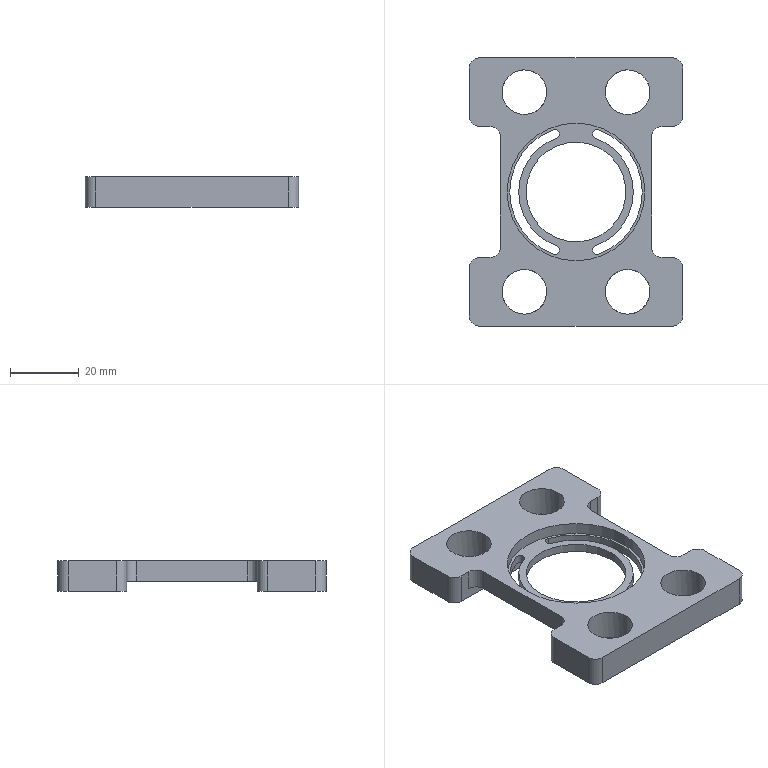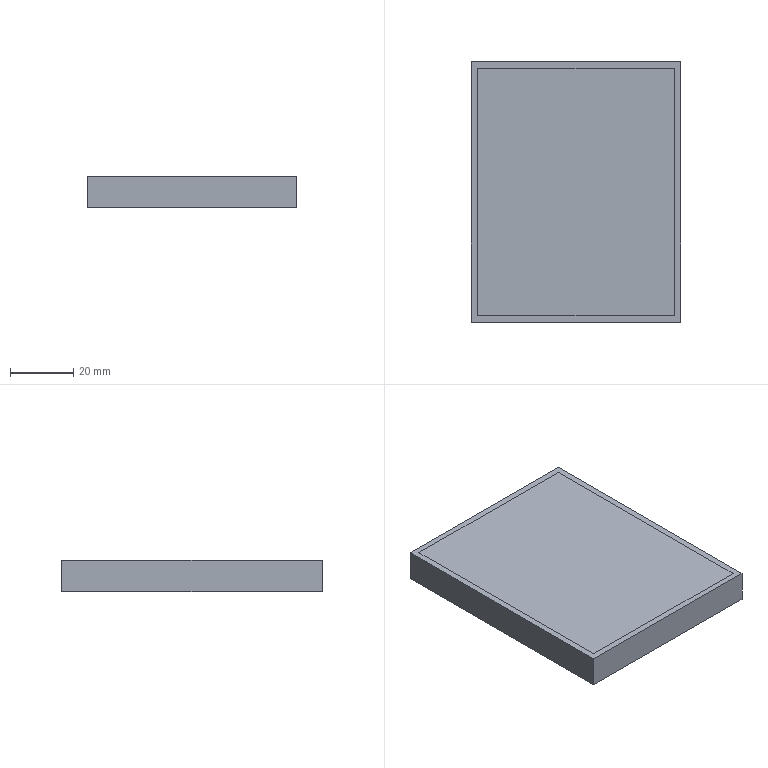CAM job | NX | 3-axis milling | part box 62 x 78 x 9 mm | stock box 66 x 82 x 10 mm
Tools:
number,name,description,diameter,corner_radius,flute_length,length,flutes
10,D10,Milling Tool-5 Parameters,10.0,0.0,50.0,75.0,2
6,D6,Milling Tool-5 Parameters,6.0,0.0,50.0,75.0,2
2,D2,Milling Tool-5 Parameters,2.0,0.0,50.0,75.0,2
7,D6A45,Milling Tool-5 Parameters,6.0,0.0,50.0,75.0,2
Operations:
program,operation,operation_type,tool,method,geometry_group,spindle_rpm,surface_speed,feed_per_tooth,feed_cut,feed_plunge,cut_length_mm,path_length_mm,cut_time_min,machine_time_min
1_GLUE,FLOOR_WALL,VolumeBased25DMillingOperation,D10,METHOD,A,9500.0,298.0,0.0658,1250.0,100.0,1361.997,1415.997,1.09,1.095
1_GLUE,HOLE_MILLING,CylinderMilling,D10,METHOD,A,9500.0,298.0,0.0658,1250.0,100.0,722.389,1114.389,0.5779,0.6171
1_GLUE,HOLE_MILLING_COPY,CylinderMilling,D10,METHOD,A,9500.0,298.0,0.0658,1250.0,100.0,1778.829,1849.829,1.423,1.43
1_GLUE,HOLE_MILLING_COPY_COPY,CylinderMilling,D10,METHOD,A,9500.0,298.0,0.0658,1250.0,100.0,664.485,736.485,0.5316,0.5388
1_GLUE,ZLEVEL_PROFILE,ZLevelMilling,D6,METHOD,A,9500.0,179.0,0.1316,2500.0,1000.0,5505.511,5570.911,2.225,2.232
1_GLUE,ZLEVEL_PROFILE_COPY,ZLevelMilling,D6,METHOD,A,9500.0,179.0,0.0526,1000.0,1000.0,329.171,1136.053,0.3292,0.4099
1_GLUE,ZLEVEL_PROFILE_COPY_COPY,ZLevelMilling,D6,METHOD,A,9500.0,179.0,0.0526,1000.0,1000.0,78.284,148.284,0.0783,0.0853
1_GLUE,ZLEVEL_PROFILE_COPY_1,ZLevelMilling,D2,METHOD,A,9500.0,179.0,0.1316,2500.0,1000.0,3129.254,3291.616,1.29,1.306
1_GLUE,PLANAR_MILL,PlanarMilling,D6A45,METHOD,A,9500.0,179.0,0.0658,1250.0,100.0,589.428,1119.535,0.4715,0.5246
1_GLUE,PLANAR_MILL_COPY,PlanarMilling,D6A45,METHOD,A,9500.0,179.0,0.0658,1250.0,100.0,89.197,156.197,0.0714,0.0781
1_GLUE,ZLEVEL_PROFILE_COPY_2,ZLevelMilling,D6,METHOD,A,9500.0,179.0,0.0632,1200.0,1000.0,1448.004,1509.304,1.232,1.239
2,FLOOR_WALL_COPY,VolumeBased25DMillingOperation,D10,METHOD,B,9500.0,298.0,0.0658,1250.0,100.0,1213.997,1267.997,0.9712,0.9766
2,FLOOR_WALL_COPY_COPY,VolumeBased25DMillingOperation,D10,METHOD,B,9500.0,298.0,0.1316,2500.0,100.0,2573.836,3300.192,1.03,1.102
2,FLOOR_WALL_COPY_COPY_COPY,VolumeBased25DMillingOperation,D10,METHOD,B,9500.0,298.0,0.0632,1200.0,100.0,581.157,816.663,0.4843,0.5078
2,PLANAR_MILL_COPY_1,PlanarMilling,D6A45,METHOD,B,9500.0,179.0,0.0658,1250.0,100.0,492.224,985.353,0.3938,0.4431
2,PLANAR_MILL_COPY_1_COPY,PlanarMilling,D6A45,METHOD,B,9500.0,179.0,0.0658,1250.0,100.0,330.464,752.414,0.2644,0.3066